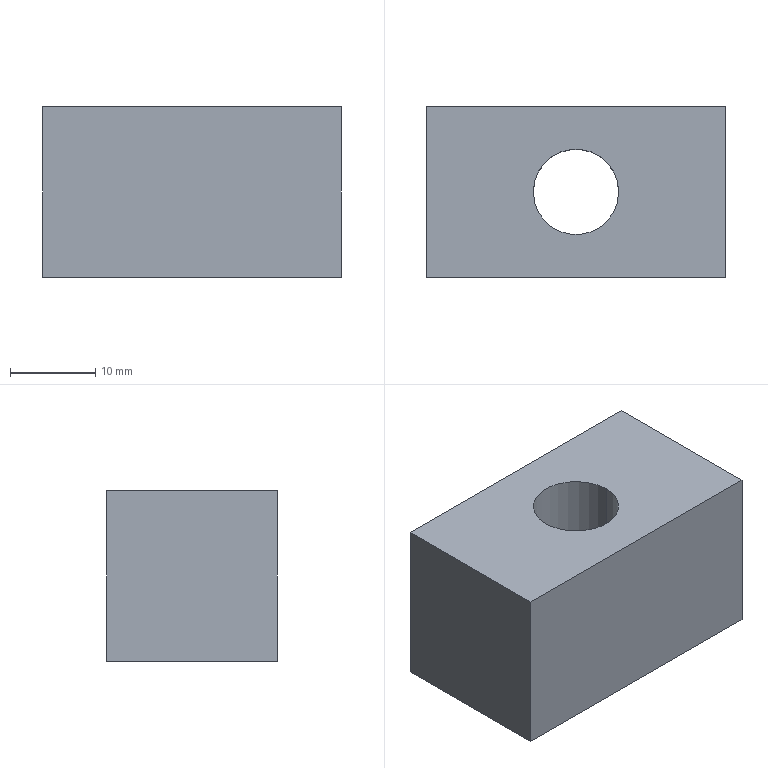Part | SolidWorks | features Extrusion 1 | 1 solid | 8 faces | box 35 x 20 x 20 mm | volume 12429 mm3 | plane 6 | cylinder 2 | commonest cylinder face diameters 10 x2
STEP:
#1=CARTESIAN_POINT('',(-5.,0.,20.));
#2=VERTEX_POINT('',#1);
#3=CARTESIAN_POINT('',(5.,0.,20.));
#4=VERTEX_POINT('',#3);
#5=CARTESIAN_POINT('',(0.,0.,20.));
#6=DIRECTION('',(0.,0.,1.));
#7=DIRECTION('',(1.,0.,0.));
#8=AXIS2_PLACEMENT_3D('',#5,#6,#7);
#9=CIRCLE('',#8,5.);
#10=EDGE_CURVE('',#2,#4,#9,.T.);
#11=ORIENTED_EDGE('',*,*,#10,.T.);
#12=CARTESIAN_POINT('',(5.,0.,0.));
#13=VERTEX_POINT('',#12);
#14=CARTESIAN_POINT('',(5.,0.,20.));
#15=DIRECTION('',(0.,0.,-1.));
#16=VECTOR('',#15,1000.);
#17=LINE('',#14,#16);
#18=EDGE_CURVE('',#4,#13,#17,.T.);
#19=ORIENTED_EDGE('',*,*,#18,.T.);
#20=CARTESIAN_POINT('',(-5.,0.,0.));
#21=VERTEX_POINT('',#20);
#22=CARTESIAN_POINT('',(0.,0.,0.));
#23=DIRECTION('',(0.,0.,1.));
#24=DIRECTION('',(1.,0.,0.));
#25=AXIS2_PLACEMENT_3D('',#22,#23,#24);
#26=CIRCLE('',#25,5.);
#27=EDGE_CURVE('',#21,#13,#26,.T.);
#28=ORIENTED_EDGE('',*,*,#27,.F.);
#29=CARTESIAN_POINT('',(-5.,0.,20.));
#30=DIRECTION('',(0.,0.,-1.));
#31=VECTOR('',#30,1000.);
#32=LINE('',#29,#31);
#33=EDGE_CURVE('',#2,#21,#32,.T.);
#34=ORIENTED_EDGE('',*,*,#33,.F.);
#35=EDGE_LOOP('',(#11,#19,#28,#34));
#36=FACE_OUTER_BOUND('',#35,.T.);
#37=CARTESIAN_POINT('',(0.,0.,20.));
#38=DIRECTION('',(0.,0.,-1.));
#39=DIRECTION('',(-1.,0.,0.));
#40=AXIS2_PLACEMENT_3D('',#37,#38,#39);
#41=CYLINDRICAL_SURFACE('',#40,5.);
#42=ADVANCED_FACE('',(#36),#41,.F.);
#43=CARTESIAN_POINT('',(17.5,-10.,20.));
#44=VERTEX_POINT('',#43);
#45=CARTESIAN_POINT('',(17.5,10.,20.));
#46=VERTEX_POINT('',#45);
#47=CARTESIAN_POINT('',(17.5,10.,20.));
#48=DIRECTION('',(0.,1.,0.));
#49=VECTOR('',#48,1000.);
#50=LINE('',#47,#49);
#51=EDGE_CURVE('',#44,#46,#50,.T.);
#52=ORIENTED_EDGE('',*,*,#51,.T.);
#53=CARTESIAN_POINT('',(-17.5,10.,20.));
#54=VERTEX_POINT('',#53);
#55=CARTESIAN_POINT('',(-17.5,10.,20.));
#56=DIRECTION('',(-1.,0.,0.));
#57=VECTOR('',#56,1000.);
#58=LINE('',#55,#57);
#59=EDGE_CURVE('',#46,#54,#58,.T.);
#60=ORIENTED_EDGE('',*,*,#59,.T.);
#61=CARTESIAN_POINT('',(-17.5,-10.,20.));
#62=VERTEX_POINT('',#61);
#63=CARTESIAN_POINT('',(-17.5,10.,20.));
#64=DIRECTION('',(0.,-1.,0.));
#65=VECTOR('',#64,1000.);
#66=LINE('',#63,#65);
#67=EDGE_CURVE('',#54,#62,#66,.T.);
#68=ORIENTED_EDGE('',*,*,#67,.T.);
#69=CARTESIAN_POINT('',(-17.5,-10.,20.));
#70=DIRECTION('',(1.,0.,0.));
#71=VECTOR('',#70,1000.);
#72=LINE('',#69,#71);
#73=EDGE_CURVE('',#62,#44,#72,.T.);
#74=ORIENTED_EDGE('',*,*,#73,.T.);
#75=EDGE_LOOP('',(#52,#60,#68,#74));
#76=FACE_OUTER_BOUND('',#75,.T.);
#77=ORIENTED_EDGE('',*,*,#10,.F.);
#78=CARTESIAN_POINT('',(0.,0.,20.));
#79=DIRECTION('',(0.,0.,1.));
#80=DIRECTION('',(1.,0.,0.));
#81=AXIS2_PLACEMENT_3D('',#78,#79,#80);
#82=CIRCLE('',#81,5.);
#83=EDGE_CURVE('',#4,#2,#82,.T.);
#84=ORIENTED_EDGE('',*,*,#83,.F.);
#85=EDGE_LOOP('',(#77,#84));
#86=FACE_BOUND('',#85,.T.);
#87=CARTESIAN_POINT('',(0.,0.,20.));
#88=DIRECTION('',(0.,0.,1.));
#89=DIRECTION('',(1.,0.,0.));
#90=AXIS2_PLACEMENT_3D('',#87,#88,#89);
#91=PLANE('',#90);
#92=ADVANCED_FACE('',(#76,#86),#91,.T.);
#93=CARTESIAN_POINT('',(17.5,-10.,0.));
#94=VERTEX_POINT('',#93);
#95=CARTESIAN_POINT('',(17.5,10.,0.));
#96=VERTEX_POINT('',#95);
#97=CARTESIAN_POINT('',(17.5,10.,0.));
#98=DIRECTION('',(0.,1.,0.));
#99=VECTOR('',#98,1000.);
#100=LINE('',#97,#99);
#101=EDGE_CURVE('',#94,#96,#100,.T.);
#102=ORIENTED_EDGE('',*,*,#101,.F.);
#103=CARTESIAN_POINT('',(-17.5,-10.,0.));
#104=VERTEX_POINT('',#103);
#105=CARTESIAN_POINT('',(-17.5,-10.,0.));
#106=DIRECTION('',(1.,0.,0.));
#107=VECTOR('',#106,1000.);
#108=LINE('',#105,#107);
#109=EDGE_CURVE('',#104,#94,#108,.T.);
#110=ORIENTED_EDGE('',*,*,#109,.F.);
#111=CARTESIAN_POINT('',(-17.5,10.,0.));
#112=VERTEX_POINT('',#111);
#113=CARTESIAN_POINT('',(-17.5,10.,0.));
#114=DIRECTION('',(0.,-1.,0.));
#115=VECTOR('',#114,1000.);
#116=LINE('',#113,#115);
#117=EDGE_CURVE('',#112,#104,#116,.T.);
#118=ORIENTED_EDGE('',*,*,#117,.F.);
#119=CARTESIAN_POINT('',(-17.5,10.,0.));
#120=DIRECTION('',(-1.,0.,0.));
#121=VECTOR('',#120,1000.);
#122=LINE('',#119,#121);
#123=EDGE_CURVE('',#96,#112,#122,.T.);
#124=ORIENTED_EDGE('',*,*,#123,.F.);
#125=EDGE_LOOP('',(#102,#110,#118,#124));
#126=FACE_OUTER_BOUND('',#125,.T.);
#127=ORIENTED_EDGE('',*,*,#27,.T.);
#128=CARTESIAN_POINT('',(0.,0.,0.));
#129=DIRECTION('',(0.,0.,1.));
#130=DIRECTION('',(1.,0.,0.));
#131=AXIS2_PLACEMENT_3D('',#128,#129,#130);
#132=CIRCLE('',#131,5.);
#133=EDGE_CURVE('',#13,#21,#132,.T.);
#134=ORIENTED_EDGE('',*,*,#133,.T.);
#135=EDGE_LOOP('',(#127,#134));
#136=FACE_BOUND('',#135,.T.);
#137=CARTESIAN_POINT('',(0.,0.,0.));
#138=DIRECTION('',(0.,0.,1.));
#139=DIRECTION('',(1.,0.,0.));
#140=AXIS2_PLACEMENT_3D('',#137,#138,#139);
#141=PLANE('',#140);
#142=ADVANCED_FACE('',(#126,#136),#141,.F.);
#143=ORIENTED_EDGE('',*,*,#101,.T.);
#144=CARTESIAN_POINT('',(17.5,10.,20.));
#145=DIRECTION('',(0.,0.,-1.));
#146=VECTOR('',#145,1000.);
#147=LINE('',#144,#146);
#148=EDGE_CURVE('',#46,#96,#147,.T.);
#149=ORIENTED_EDGE('',*,*,#148,.F.);
#150=ORIENTED_EDGE('',*,*,#51,.F.);
#151=CARTESIAN_POINT('',(17.5,-10.,20.));
#152=DIRECTION('',(0.,0.,-1.));
#153=VECTOR('',#152,1000.);
#154=LINE('',#151,#153);
#155=EDGE_CURVE('',#44,#94,#154,.T.);
#156=ORIENTED_EDGE('',*,*,#155,.T.);
#157=EDGE_LOOP('',(#143,#149,#150,#156));
#158=FACE_OUTER_BOUND('',#157,.T.);
#159=CARTESIAN_POINT('',(17.5,10.,20.));
#160=DIRECTION('',(-1.,0.,0.));
#161=DIRECTION('',(0.,-1.,0.));
#162=AXIS2_PLACEMENT_3D('',#159,#160,#161);
#163=PLANE('',#162);
#164=ADVANCED_FACE('',(#158),#163,.F.);
#165=ORIENTED_EDGE('',*,*,#123,.T.);
#166=CARTESIAN_POINT('',(-17.5,10.,20.));
#167=DIRECTION('',(0.,0.,-1.));
#168=VECTOR('',#167,1000.);
#169=LINE('',#166,#168);
#170=EDGE_CURVE('',#54,#112,#169,.T.);
#171=ORIENTED_EDGE('',*,*,#170,.F.);
#172=ORIENTED_EDGE('',*,*,#59,.F.);
#173=ORIENTED_EDGE('',*,*,#148,.T.);
#174=EDGE_LOOP('',(#165,#171,#172,#173));
#175=FACE_OUTER_BOUND('',#174,.T.);
#176=CARTESIAN_POINT('',(-17.5,10.,20.));
#177=DIRECTION('',(0.,-1.,0.));
#178=DIRECTION('',(0.,0.,-1.));
#179=AXIS2_PLACEMENT_3D('',#176,#177,#178);
#180=PLANE('',#179);
#181=ADVANCED_FACE('',(#175),#180,.F.);
#182=ORIENTED_EDGE('',*,*,#117,.T.);
#183=CARTESIAN_POINT('',(-17.5,-10.,20.));
#184=DIRECTION('',(0.,0.,-1.));
#185=VECTOR('',#184,1000.);
#186=LINE('',#183,#185);
#187=EDGE_CURVE('',#62,#104,#186,.T.);
#188=ORIENTED_EDGE('',*,*,#187,.F.);
#189=ORIENTED_EDGE('',*,*,#67,.F.);
#190=ORIENTED_EDGE('',*,*,#170,.T.);
#191=EDGE_LOOP('',(#182,#188,#189,#190));
#192=FACE_OUTER_BOUND('',#191,.T.);
#193=CARTESIAN_POINT('',(-17.5,10.,20.));
#194=DIRECTION('',(1.,0.,0.));
#195=DIRECTION('',(0.,1.,0.));
#196=AXIS2_PLACEMENT_3D('',#193,#194,#195);
#197=PLANE('',#196);
#198=ADVANCED_FACE('',(#192),#197,.F.);
#199=ORIENTED_EDGE('',*,*,#109,.T.);
#200=ORIENTED_EDGE('',*,*,#155,.F.);
#201=ORIENTED_EDGE('',*,*,#73,.F.);
#202=ORIENTED_EDGE('',*,*,#187,.T.);
#203=EDGE_LOOP('',(#199,#200,#201,#202));
#204=FACE_OUTER_BOUND('',#203,.T.);
#205=CARTESIAN_POINT('',(-17.5,-10.,20.));
#206=DIRECTION('',(0.,1.,0.));
#207=DIRECTION('',(0.,0.,1.));
#208=AXIS2_PLACEMENT_3D('',#205,#206,#207);
#209=PLANE('',#208);
#210=ADVANCED_FACE('',(#204),#209,.F.);
#211=ORIENTED_EDGE('',*,*,#18,.F.);
#212=ORIENTED_EDGE('',*,*,#83,.T.);
#213=ORIENTED_EDGE('',*,*,#33,.T.);
#214=ORIENTED_EDGE('',*,*,#133,.F.);
#215=EDGE_LOOP('',(#211,#212,#213,#214));
#216=FACE_OUTER_BOUND('',#215,.T.);
#217=CARTESIAN_POINT('',(0.,0.,20.));
#218=DIRECTION('',(0.,0.,-1.));
#219=DIRECTION('',(-1.,0.,0.));
#220=AXIS2_PLACEMENT_3D('',#217,#218,#219);
#221=CYLINDRICAL_SURFACE('',#220,5.);
#222=ADVANCED_FACE('',(#216),#221,.F.);
#223=CLOSED_SHELL('',(#42,#92,#142,#164,#181,#198,#210,#222));
#224=MANIFOLD_SOLID_BREP('',#223);
#225=CARTESIAN_POINT('',(0.,0.,0.));
#226=DIRECTION('',(0.,0.,1.));
#227=DIRECTION('',(1.,0.,0.));
#228=AXIS2_PLACEMENT_3D('',#225,#226,#227);
#229=(LENGTH_UNIT()NAMED_UNIT(*)SI_UNIT(.MILLI.,.METRE.));
#230=UNCERTAINTY_MEASURE_WITH_UNIT(LENGTH_MEASURE(0.00001),#229,'','');
#231=(NAMED_UNIT(*)PLANE_ANGLE_UNIT()SI_UNIT($,.RADIAN.));
#232=(NAMED_UNIT(*)SI_UNIT($,.STERADIAN.)SOLID_ANGLE_UNIT());
#233=(GEOMETRIC_REPRESENTATION_CONTEXT(3)GLOBAL_UNCERTAINTY_ASSIGNED_CONTEXT((#230))GLOBAL_UNIT_ASSIGNED_CONTEXT((#229,#231,#232))REPRESENTATION_CONTEXT('',''));
#234=ADVANCED_BREP_SHAPE_REPRESENTATION('',(#224,#228),#233);